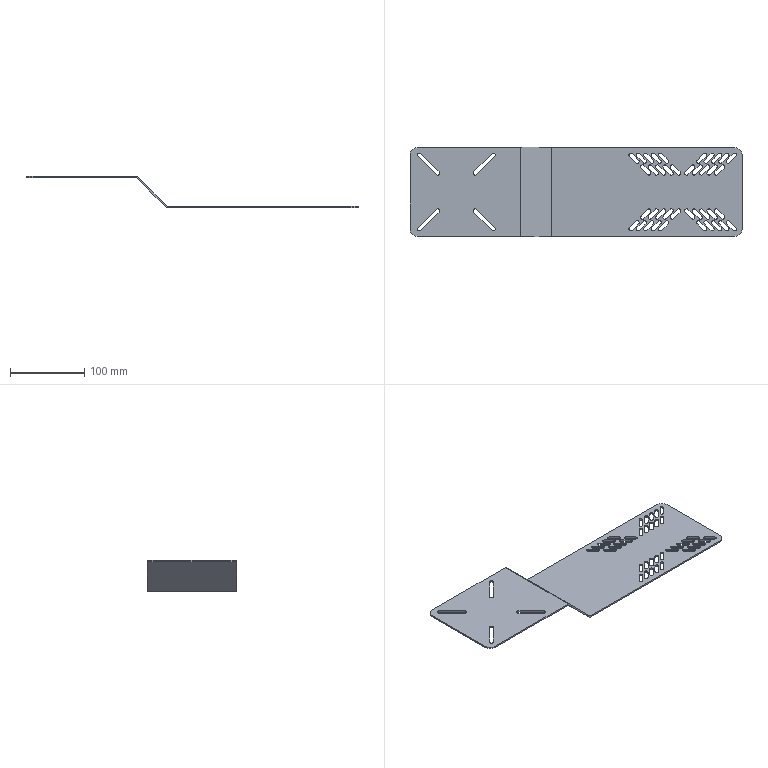Part | STEP file | 1 solid | 194 faces | box 447.598 x 120 x 42.426 mm | volume 103118 mm3 | plane 98 | cylinder 96 | commonest cylinder face diameters 5 x88 20 x4 0.4 x2 4.4 x2